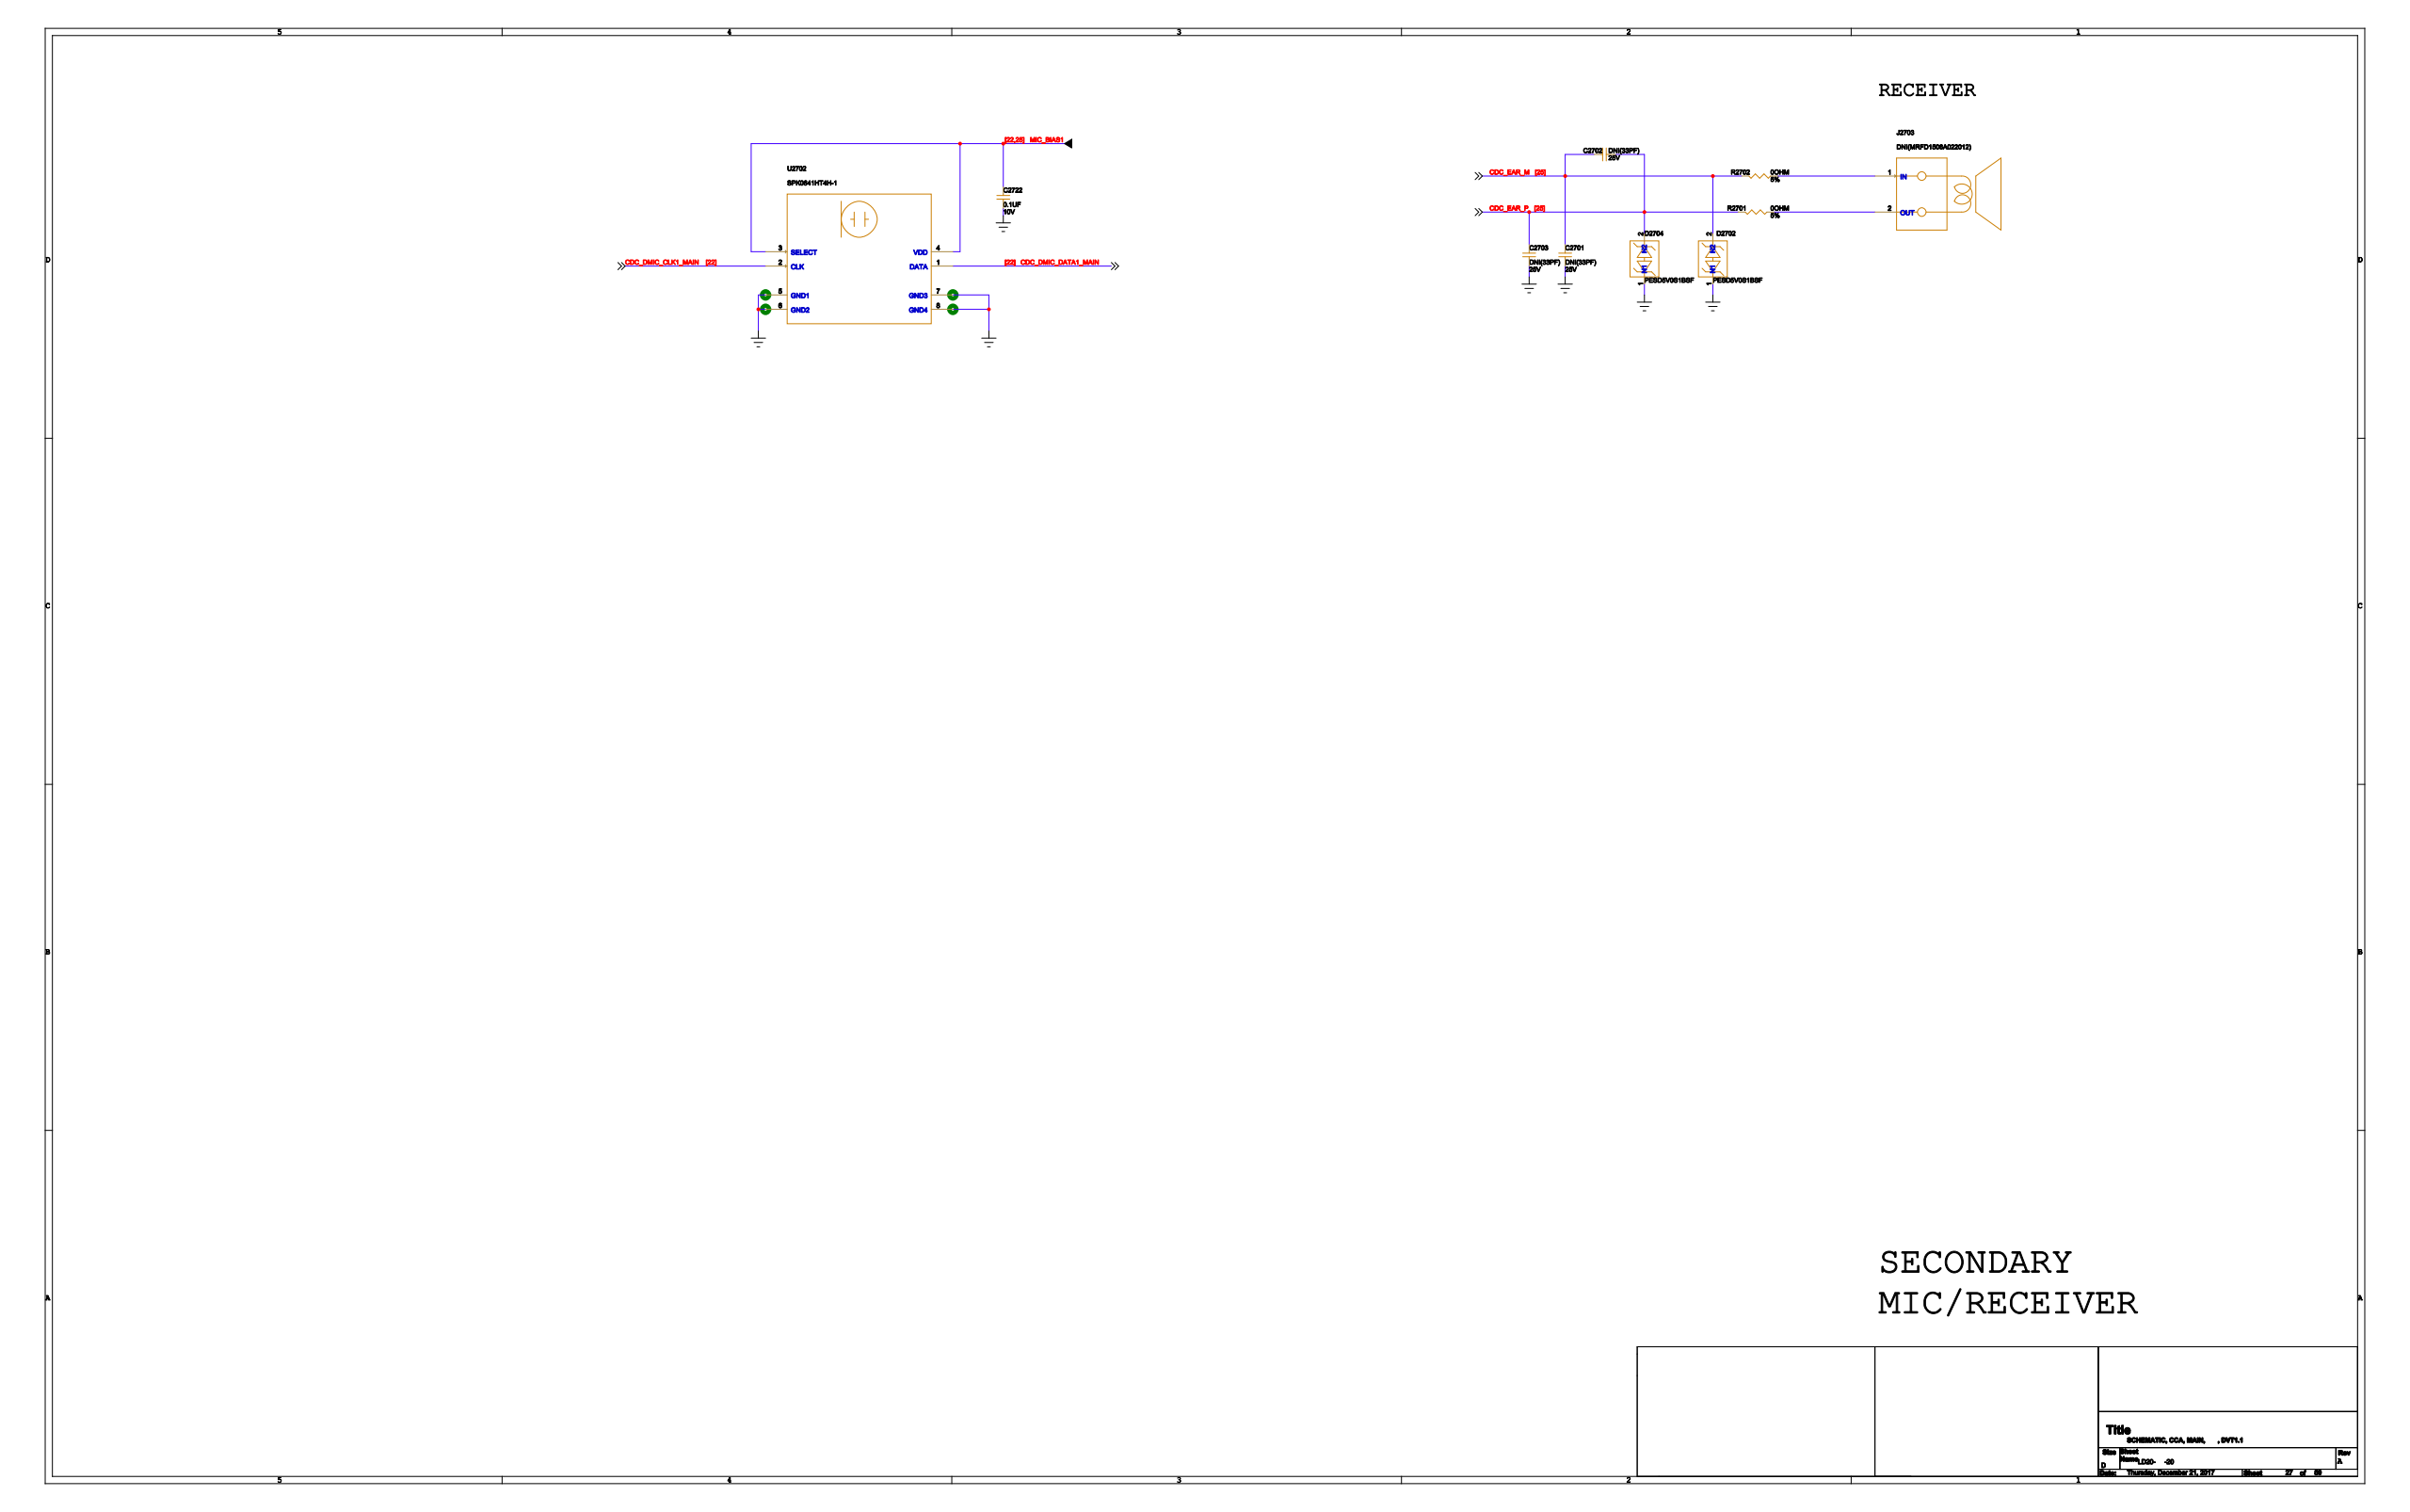Circuit board | Cadence Allegro | 1520 parts | 1149 nets | one sheet of the schematic
Parts on this sheet (reference | value | footprint):
C2701 | DNI(33PF) | 2P0201R_DNI
C2702 | DNI(33PF) | 2P0201R_DNI
C2703 | DNI(33PF) | 2P0201R_DNI
C2722 | 0.1UF | 2P0201R
D2702 | PESD5V0S1BSF | 2PSM25X13N
D2704 | PESD5V0S1BSF | 2PSM25X13N
J2703 | DNI(MRFD1506A022012) | MRFD1506A022012_DNI
R2701 | 0OHM | 2P0402R
R2702 | 0OHM | 2P0402R
U2702 | SPK0641HT4H-1 | 8PSM161X122NV3
Nets of these parts (net: part-pin ...):
GND: C2701-2 C2703-2 C2722-2 D2702-1 D2704-1 U2702-5 U2702-6 U2702-7 U2702-8
N21133399: J2703-1 R2702-2
N21133402: J2703-2 R2701-2
MIC_BIAS1: C2722-1 U2702-3 U2702-4
CDC_DMIC_CLK1_MAIN: U2702-2
CDC_DMIC_DATA1_MAIN: U2702-1
CDC_EAR_M: C2701-1 C2702-1 D2702-2 R2702-1
CDC_EAR_P: C2702-2 C2703-1 D2704-2 R2701-1